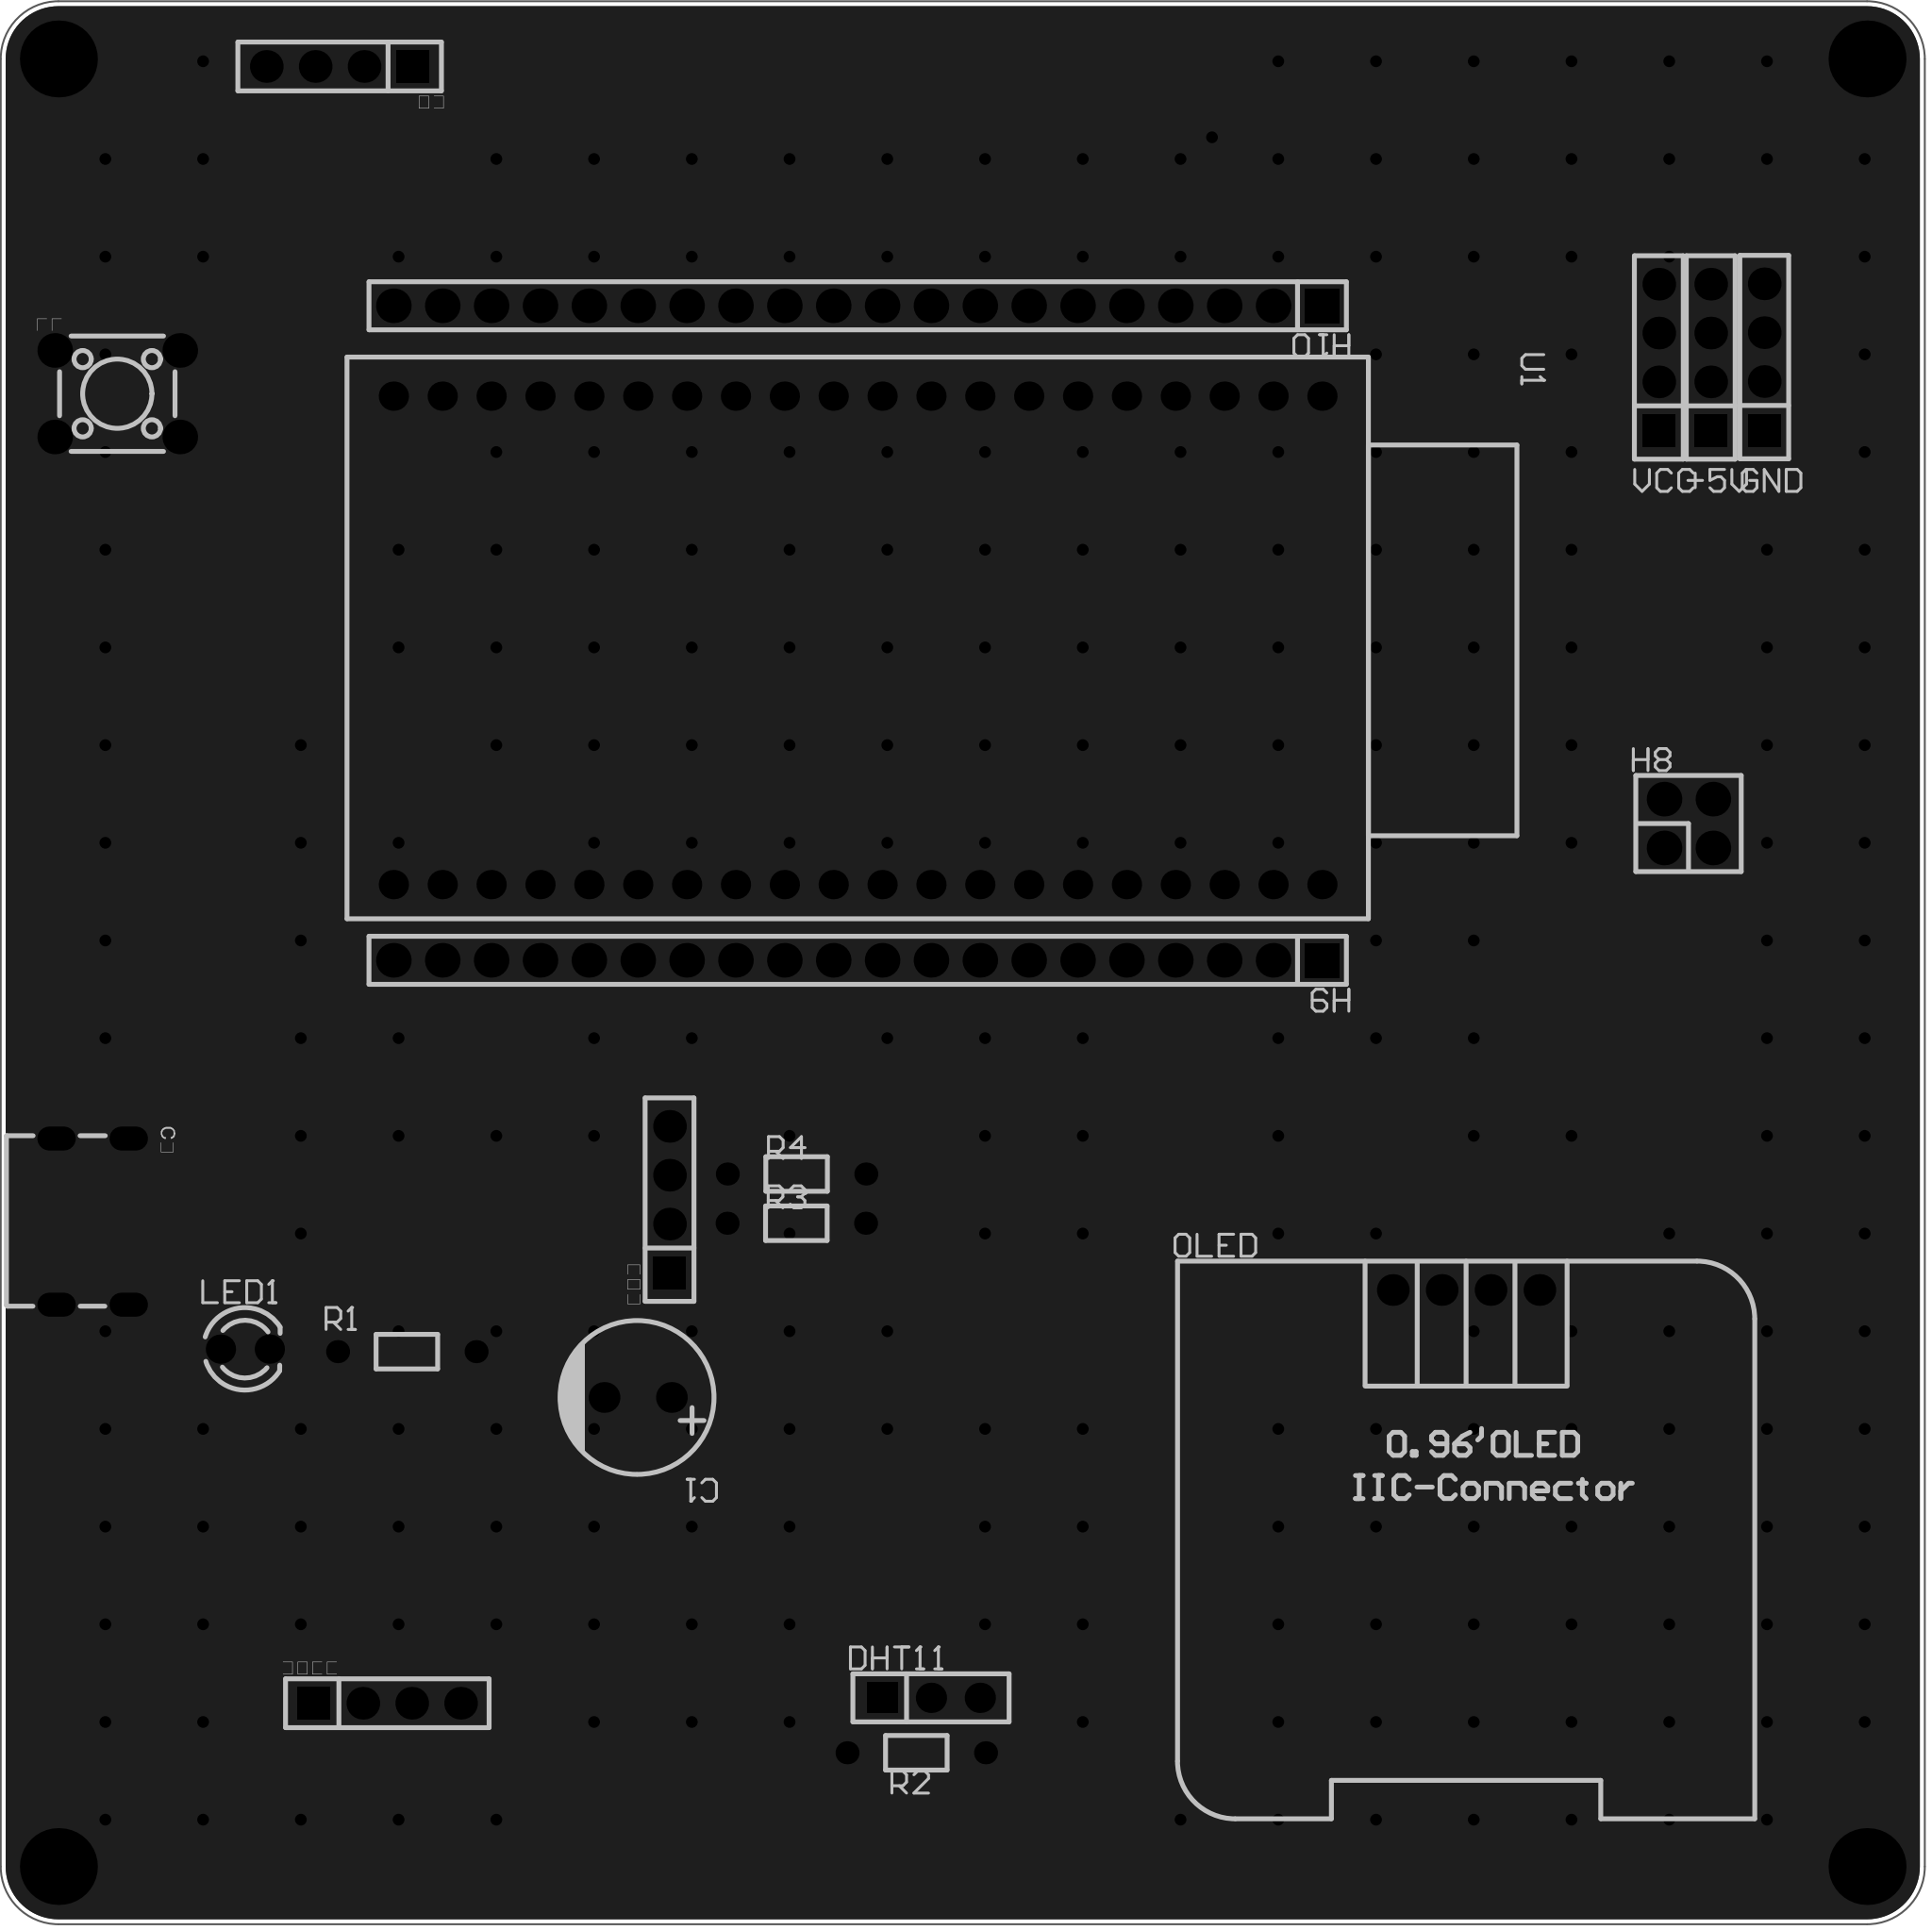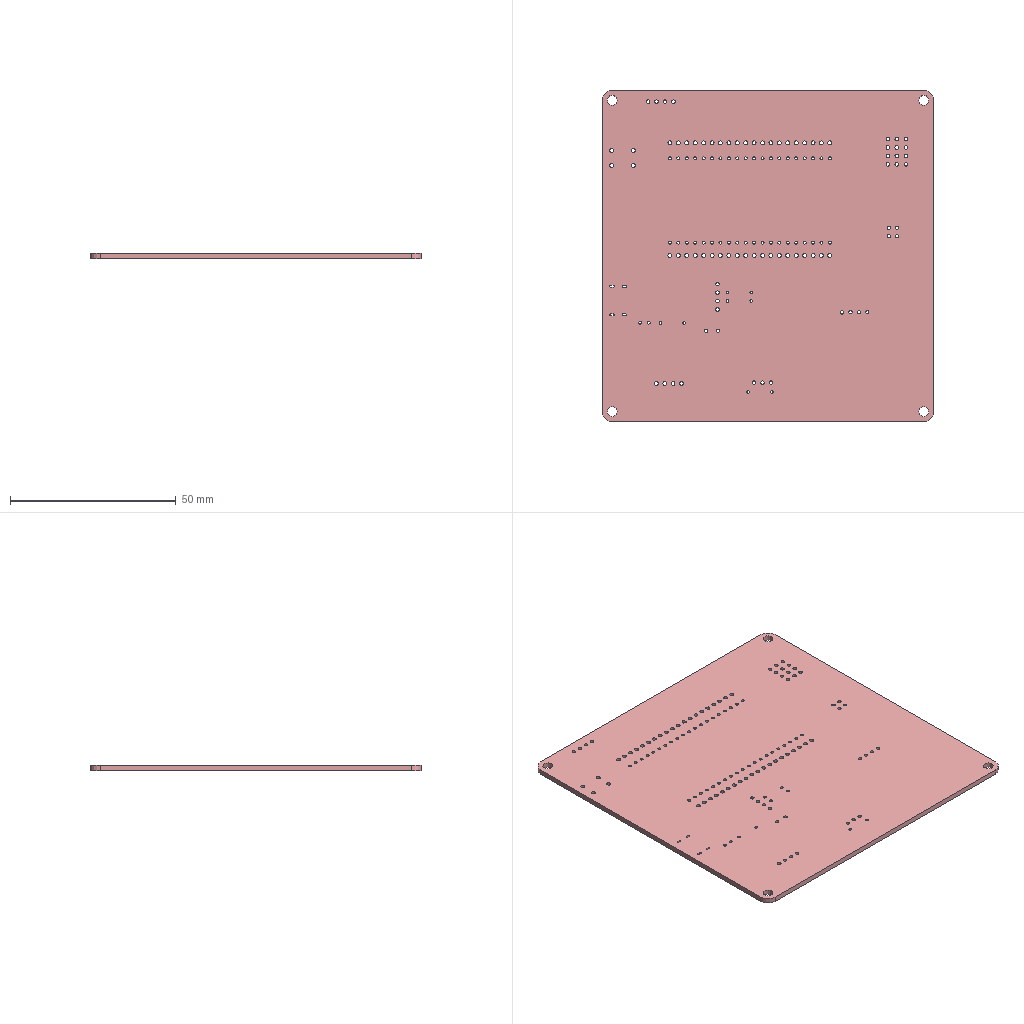Circuit board layout | Altium Designer | box 100 x 100 x 1.6 mm
Layer stack:
# Altium Designer layer stack of  (unit mm; dielectric type: 0 none, 1 core, 2 prepreg, 3 surface material)
index,name,kind,layer,copper_thickness_mm,dielectric_type,dielectric_thickness_mm,dielectric_material,dielectric_constant
0,Top Paste Mask Layer,other,,,,,,
1,Top Silkscreen Layer,other,,,,,,
2,Top Solder Mask Layer,dielectric,,,3,0.01,,3.3
3,Top Layer,copper,Top Layer,0.035,,,,
4,Dielectric1,dielectric,,,3,1.51,FR4,4.5
5,Bottom Layer,copper,Bottom Layer,0.035,,,,
6,Bottom Solder Mask Layer,dielectric,,,3,0.01,,3.3
7,Bottom Silkscreen Layer,other,,,,,,
8,Bottom Paste Mask Layer,other,,,,,,
# drill layer pairs: low layer,high layer
drill_pair,Top Layer,Bottom Layer
Part placement:
Designator,Comment,Layer,Footprint,Center-X(mm),Center-Y(mm),Rotation
DHT11,,TopLayer,HDR-TH_3P-P2.54-V-F,139.7,92.71,0
光敏电阻,,TopLayer,HDR-TH_4P-P2.54-V-F,111.443,92.43,0
OLED,,TopLayer,0.96OLED_4P,167.513,113.919,0
R1,220Ω,TopLayer,Res_1/8W,112.459,110.713,0
+5V,,TopLayer,HDR-TH_4P-P2.54-V-F,180.226,162.414,90
C1,100uF,TopLayer,CAP-TH_BD8.0-P3.50-D0.6-FD_1,124.46,108.331,180
C?,,TopLayer,USB__TYPE-C-6P,96.393,117.475,270
GND,,TopLayer,HDR-TH_4P-P2.54-V-F,183.007,162.433,90
H8,,TopLayer,HDR-TH_4P-P2.54-V-F-R2-C2-S2.54,179.07,138.176,0
H9,,TopLayer,HDR-TH_20P-P2.54-V-M-1,135.89,131.064,180
H10,,TopLayer,HDR-TH_20P-P2.54-V-M-1,135.89,165.1,180
VCC,,TopLayer,HDR-TH_4P-P2.54-V-F,177.528,162.414,90
容珊尺,,TopLayer,HDR-TH_4P-P2.54-V-F,126.111,118.618,90
按键,,TopLayer,SW-TH_4P-L6.0-W6.0-P4.50-LS6.5,97.409,160.528,0
电机,,TopLayer,HDR-TH_4P-P2.54-V-F,108.966,177.546,180
LED1,,TopLayer,LED_TH-3mm,104.043,110.845,0
U1,,TopLayer,ESP32-S3-CAM,135.89,147.701,270
R2,4.7K,TopLayer,Res_1/8W,138.938,89.853,180
R3,4.7K,TopLayer,Res_1/8W,132.702,117.39,0
R4,4.7K,TopLayer,Res_1/8W,132.715,119.951,0
Pad and via stacks:
# Altium Designer via and pad stacks of  (unit mm). Each distinct definition once, with the count of objects using it.
# via: kind,start_layer,end_layer,hole_mm,diameter_mm,mode(0 simple;1 top-mid-bottom;2 full stack),diameter_per_layer,count,example_net
# pad: kind,layer,hole_mm,hole_type(0 round;1 square;2 slot),plating,top_size,top_shape(1 round;2 rect;3 octagon;9 rounded rect),mid_size,bottom_size,mode,footprint,size_per_layer,count,example
pad,Multi-Layer,3,0,plated,4x4,1,4x4,4x4,0,,,4,1
pad,Multi-Layer,1.02,0,plated,1.575x1.575,1,1.575x1.575,1.575x1.575,0,HDR-TH_3P-P2.54-V-F,,2,DHT11.3
pad,Multi-Layer,1.02,0,plated,1.575x1.575,2,1.575x1.575,1.575x1.575,0,HDR-TH_3P-P2.54-V-F,,1,DHT11.1
pad,Multi-Layer,1.1,0,plated,1.7x1.7,2,1.7x1.7,1.7x1.7,0,HDR-TH_4P-P2.54-V-F,,6,\u5149\u654F\u7535\u963B.1
pad,Multi-Layer,1.1,0,plated,1.7x1.7,1,1.7x1.7,1.7x1.7,0,HDR-TH_4P-P2.54-V-F,,18,\u5149\u654F\u7535\u963B.2
pad,Multi-Layer,1,0,plated,1.65x1.65,1,1.65x1.65,1.65x1.65,0,0.96OLED_4P,,4,OLED.4
pad,Multi-Layer,0.8001,0,plated,1.199x1.199,1,1.199x1.199,1.199x1.199,0,Res_1/8W,,8,R1.1
pad,Multi-Layer,1,0,plated,1.6x1.6,1,1.6x1.6,1.6x1.6,0,CAP-TH_BD8.0-P3.50-D0.6-FD_1,,2,C1.2
pad,Multi-Layer,0.6,2,plated,1.25x2,1,1.25x2,1.25x2,0,USB_ TYPE-C-6P,,4,C\u53E3.8
pad,Multi-Layer,1,0,plated,1.8x1.8,1,1.8x1.8,1.8x1.8,0,HDR-TH_4P-P2.54-V-F-R2-C2-S2.54,,4,H8.4
pad,Multi-Layer,1.2,0,plated,1.8x1.8,1,1.8x1.8,1.8x1.8,0,HDR-TH_20P-P2.54-V-M-1,,38,H9.20
pad,Multi-Layer,1.2,0,plated,1.8x1.8,2,1.8x1.8,1.8x1.8,0,HDR-TH_20P-P2.54-V-M-1,,2,H9.1
pad,Multi-Layer,1.2,0,plated,1.8x1.8,1,1.8x1.8,1.8x1.8,0,SW-TH_4P-L6.0-W6.0-P4.50-LS6.5,,4,\u6309\u952E.1
pad,Multi-Layer,0.9144,0,plated,1.524x1.524,1,1.524x1.524,1.524x1.524,0,LED_TH-3mm,,2,LED1.1
pad,Multi-Layer,0.9144,0,plated,1.524x1.524,1,1.524x1.524,1.524x1.524,0,ESP32-S3-CAM,,40,U1.2
pad,Top Layer,0,0,plated,0.7x1.2,2,0.7x1.2,0.7x1.2,0,USB_ TYPE-C-6P,,2,C\u53E3.A5
pad,Top Layer,0,0,plated,0.8x1.2,2,0.8x1.2,0.8x1.2,0,USB_ TYPE-C-6P,,2,C\u53E3.B9
pad,Top Layer,0,0,plated,0.9x1.2,2,0.9x1.2,0.9x1.2,0,USB_ TYPE-C-6P,,2,C\u53E3.B12
via,Top Layer,Bottom Layer,0.3048,0.61,0,,254,4
Copper pours:
name,layer,net,type(0 solid;1 hatched;2 none)
Bottom Layer-GND,Bottom Layer,GND,0
Top Layer-GND,Top Layer,GND,0
Design rules, without the lines most boards share:
# Altium Designer design rules of  (exported by Altium Designer, unit mm)
# columns: name | kind | enabled | priority | scope1 | scope2 | descriptor | typed fields (field=value)
Copper_copperRegion_copperThickness1oz | 0 | disabled | 4 | All | All | Clearance Constraint (Gap=5.984mil) (Disabled)(All),(All) | gap=0.152
Copper_copperRegion_copperThickness1oz_1 | 63 | disabled | 4 | All | All | Board Clearance Constraint (Gap=0mil) (Disabled)(All) |
Copper_copperRegion_Copper_copperRegion | 0 | disabled | 5 | All | All | Clearance Constraint (Gap=5.984mil) (Disabled)(All),(All) | gap=0.152
Copper_copperRegion_Copper_copperRegion_1 | 63 | disabled | 5 | All | All | Board Clearance Constraint (Gap=0mil) (Disabled)(All) |
copperThickness1oz | 0 | enabled | 6 | All | All | Clearance Constraint (Gap=5.984mil) (All),(All) | gap=0.152
copperThickness1oz_1 | 63 | enabled | 6 | All | All | Board Clearance Constraint (Gap=0mil) (All) |
copperRegion_copperThickness1oz | 20 | disabled | 1 | All | All | Polygon Connect Rule(Relief Connect )(Conductor Width=10mil) (Relief Angle=90 Angle) (Entries=4) (Air Gap Width=10mil) (Disabled)(All),(All) | connect_style(0=relief,1=direct,2=none)=0 relief_conductor_width=0.254 relief_entries=4
copperRegion_Copper_copperRegion | 20 | disabled | 2 | All | All | Polygon Connect Rule(Relief Connect )(Conductor Width=10mil) (Relief Angle=90 Angle) (Entries=4) (Air Gap Width=10mil) (Disabled)(All),(All) | connect_style(0=relief,1=direct,2=none)=0 relief_conductor_width=0.254 relief_entries=4
copperRegion | 20 | enabled | 3 | All | All | Polygon Connect Rule(Relief Connect )(Conductor Width=10mil) (Relief Angle=90 Angle) (Entries=4) (Air Gap Width=10mil) (All),(All) | connect_style(0=relief,1=direct,2=none)=0 relief_conductor_width=0.254 relief_entries=4